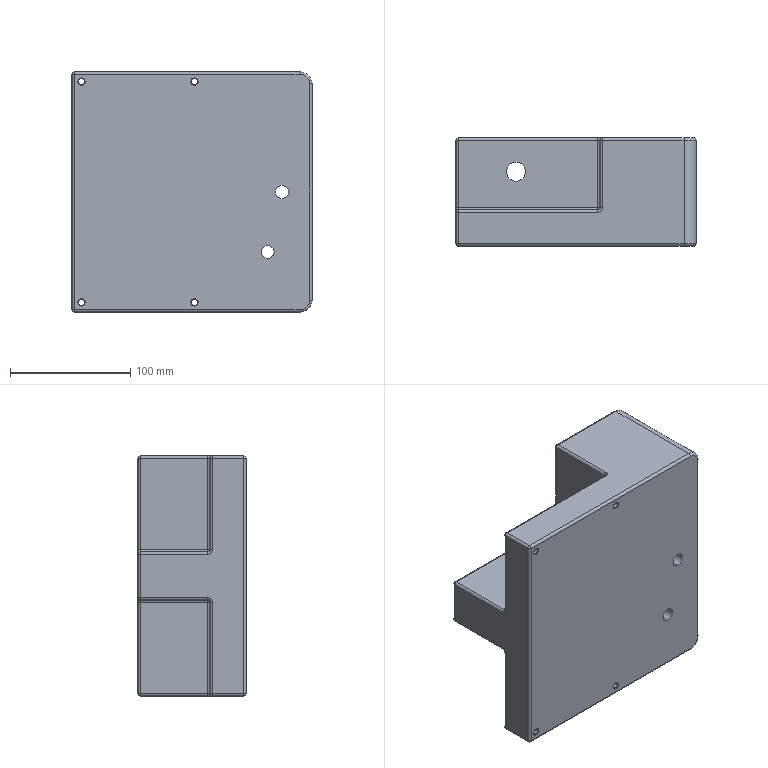Part | SolidWorks | features ICE 7, Fillet 2, Extrusion 1, HoleWzd 1, MoveFace 1 | 1 solid | 94 faces | box 200 x 90 x 200 mm | volume 2319927 mm3 | cylinder 52 | plane 14 | torus 10 | sphere 10 | cone 8 | commonest cylinder face diameters 4 x28 5 x8 11 x8 16 x2 20 x2 31 x2